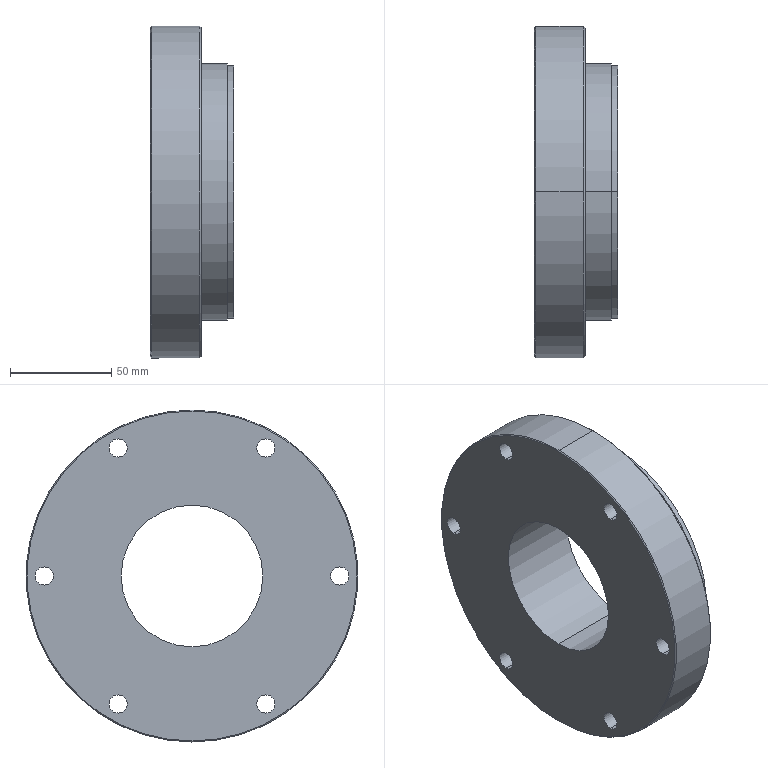Part | SolidWorks | features BaseBody 1 | 1 solid | 46 faces | box 41 x 164 x 164 mm | volume 556620 mm3 | cylinder 32 | plane 10 | cone 4 | commonest cylinder face diameters 9 x12 14 x12 70 x2 125 x2 127 x2 164 x2
STEP:
#1=CARTESIAN_POINT('',(41.,0.,-35.));
#2=VERTEX_POINT('',#1);
#3=CARTESIAN_POINT('',(41.,0.,35.));
#4=VERTEX_POINT('',#3);
#5=CARTESIAN_POINT('',(41.,0.,0.));
#6=DIRECTION('',(-1.,0.,0.));
#7=DIRECTION('',(0.,0.,1.));
#8=AXIS2_PLACEMENT_3D('',#5,#6,#7);
#9=CIRCLE('',#8,35.);
#10=EDGE_CURVE('',#2,#4,#9,.T.);
#11=ORIENTED_EDGE('',*,*,#10,.F.);
#12=CARTESIAN_POINT('',(0.,0.,-35.));
#13=VERTEX_POINT('',#12);
#14=CARTESIAN_POINT('',(-14.652,0.,-35.));
#15=DIRECTION('',(-1.,0.,0.));
#16=VECTOR('',#15,1000.);
#17=LINE('',#14,#16);
#18=EDGE_CURVE('',#2,#13,#17,.T.);
#19=ORIENTED_EDGE('',*,*,#18,.T.);
#20=CARTESIAN_POINT('',(0.,0.,35.));
#21=VERTEX_POINT('',#20);
#22=CARTESIAN_POINT('',(0.,0.,0.));
#23=DIRECTION('',(-1.,0.,0.));
#24=DIRECTION('',(0.,0.,1.));
#25=AXIS2_PLACEMENT_3D('',#22,#23,#24);
#26=CIRCLE('',#25,35.);
#27=EDGE_CURVE('',#13,#21,#26,.T.);
#28=ORIENTED_EDGE('',*,*,#27,.T.);
#29=CARTESIAN_POINT('',(-14.652,0.,35.));
#30=DIRECTION('',(-1.,0.,0.));
#31=VECTOR('',#30,1000.);
#32=LINE('',#29,#31);
#33=EDGE_CURVE('',#4,#21,#32,.T.);
#34=ORIENTED_EDGE('',*,*,#33,.F.);
#35=EDGE_LOOP('',(#11,#19,#28,#34));
#36=FACE_OUTER_BOUND('',#35,.T.);
#37=CARTESIAN_POINT('',(-14.652,0.,0.));
#38=DIRECTION('',(-1.,0.,0.));
#39=DIRECTION('',(0.,0.,1.));
#40=AXIS2_PLACEMENT_3D('',#37,#38,#39);
#41=CYLINDRICAL_SURFACE('',#40,35.);
#42=ADVANCED_FACE('',(#36),#41,.F.);
#43=CARTESIAN_POINT('',(0.,73.,-4.5));
#44=VERTEX_POINT('',#43);
#45=CARTESIAN_POINT('',(0.,73.,4.5));
#46=VERTEX_POINT('',#45);
#47=CARTESIAN_POINT('',(0.,73.,0.));
#48=DIRECTION('',(-1.,0.,0.));
#49=DIRECTION('',(0.,0.,-1.));
#50=AXIS2_PLACEMENT_3D('',#47,#48,#49);
#51=CIRCLE('',#50,4.5);
#52=EDGE_CURVE('',#44,#46,#51,.T.);
#53=ORIENTED_EDGE('',*,*,#52,.T.);
#54=CARTESIAN_POINT('',(15.,73.,4.5));
#55=VERTEX_POINT('',#54);
#56=CARTESIAN_POINT('',(25.,73.,4.5));
#57=DIRECTION('',(1.,0.,0.));
#58=VECTOR('',#57,1000.);
#59=LINE('',#56,#58);
#60=EDGE_CURVE('',#46,#55,#59,.T.);
#61=ORIENTED_EDGE('',*,*,#60,.T.);
#62=CARTESIAN_POINT('',(15.,73.,-4.5));
#63=VERTEX_POINT('',#62);
#64=CARTESIAN_POINT('',(15.,73.,0.));
#65=DIRECTION('',(-1.,0.,0.));
#66=DIRECTION('',(0.,0.,-1.));
#67=AXIS2_PLACEMENT_3D('',#64,#65,#66);
#68=CIRCLE('',#67,4.5);
#69=EDGE_CURVE('',#63,#55,#68,.T.);
#70=ORIENTED_EDGE('',*,*,#69,.F.);
#71=CARTESIAN_POINT('',(25.,73.,-4.5));
#72=DIRECTION('',(1.,0.,0.));
#73=VECTOR('',#72,1000.);
#74=LINE('',#71,#73);
#75=EDGE_CURVE('',#44,#63,#74,.T.);
#76=ORIENTED_EDGE('',*,*,#75,.F.);
#77=EDGE_LOOP('',(#53,#61,#70,#76));
#78=FACE_OUTER_BOUND('',#77,.T.);
#79=CARTESIAN_POINT('',(25.,73.,0.));
#80=DIRECTION('',(1.,0.,0.));
#81=DIRECTION('',(0.,0.,-1.));
#82=AXIS2_PLACEMENT_3D('',#79,#80,#81);
#83=CYLINDRICAL_SURFACE('',#82,4.5);
#84=ADVANCED_FACE('',(#78),#83,.F.);
#85=CARTESIAN_POINT('',(0.,36.5,-67.72));
#86=VERTEX_POINT('',#85);
#87=CARTESIAN_POINT('',(0.,36.5,-58.72));
#88=VERTEX_POINT('',#87);
#89=CARTESIAN_POINT('',(0.,36.5,-63.22));
#90=DIRECTION('',(-1.,0.,0.));
#91=DIRECTION('',(0.,0.,-1.));
#92=AXIS2_PLACEMENT_3D('',#89,#90,#91);
#93=CIRCLE('',#92,4.5);
#94=EDGE_CURVE('',#86,#88,#93,.T.);
#95=ORIENTED_EDGE('',*,*,#94,.T.);
#96=CARTESIAN_POINT('',(15.,36.5,-58.72));
#97=VERTEX_POINT('',#96);
#98=CARTESIAN_POINT('',(25.,36.5,-58.72));
#99=DIRECTION('',(1.,0.,0.));
#100=VECTOR('',#99,1000.);
#101=LINE('',#98,#100);
#102=EDGE_CURVE('',#88,#97,#101,.T.);
#103=ORIENTED_EDGE('',*,*,#102,.T.);
#104=CARTESIAN_POINT('',(15.,36.5,-67.72));
#105=VERTEX_POINT('',#104);
#106=CARTESIAN_POINT('',(15.,36.5,-63.22));
#107=DIRECTION('',(-1.,0.,0.));
#108=DIRECTION('',(0.,0.,-1.));
#109=AXIS2_PLACEMENT_3D('',#106,#107,#108);
#110=CIRCLE('',#109,4.5);
#111=EDGE_CURVE('',#105,#97,#110,.T.);
#112=ORIENTED_EDGE('',*,*,#111,.F.);
#113=CARTESIAN_POINT('',(25.,36.5,-67.72));
#114=DIRECTION('',(1.,0.,0.));
#115=VECTOR('',#114,1000.);
#116=LINE('',#113,#115);
#117=EDGE_CURVE('',#86,#105,#116,.T.);
#118=ORIENTED_EDGE('',*,*,#117,.F.);
#119=EDGE_LOOP('',(#95,#103,#112,#118));
#120=FACE_OUTER_BOUND('',#119,.T.);
#121=CARTESIAN_POINT('',(25.,36.5,-63.22));
#122=DIRECTION('',(1.,0.,0.));
#123=DIRECTION('',(0.,0.,-1.));
#124=AXIS2_PLACEMENT_3D('',#121,#122,#123);
#125=CYLINDRICAL_SURFACE('',#124,4.5);
#126=ADVANCED_FACE('',(#120),#125,.F.);
#127=CARTESIAN_POINT('',(0.,-36.5,-67.72));
#128=VERTEX_POINT('',#127);
#129=CARTESIAN_POINT('',(0.,-36.5,-58.72));
#130=VERTEX_POINT('',#129);
#131=CARTESIAN_POINT('',(0.,-36.5,-63.22));
#132=DIRECTION('',(-1.,0.,0.));
#133=DIRECTION('',(0.,0.,-1.));
#134=AXIS2_PLACEMENT_3D('',#131,#132,#133);
#135=CIRCLE('',#134,4.5);
#136=EDGE_CURVE('',#128,#130,#135,.T.);
#137=ORIENTED_EDGE('',*,*,#136,.T.);
#138=CARTESIAN_POINT('',(15.,-36.5,-58.72));
#139=VERTEX_POINT('',#138);
#140=CARTESIAN_POINT('',(25.,-36.5,-58.72));
#141=DIRECTION('',(1.,0.,0.));
#142=VECTOR('',#141,1000.);
#143=LINE('',#140,#142);
#144=EDGE_CURVE('',#130,#139,#143,.T.);
#145=ORIENTED_EDGE('',*,*,#144,.T.);
#146=CARTESIAN_POINT('',(15.,-36.5,-67.72));
#147=VERTEX_POINT('',#146);
#148=CARTESIAN_POINT('',(15.,-36.5,-63.22));
#149=DIRECTION('',(-1.,0.,0.));
#150=DIRECTION('',(0.,0.,-1.));
#151=AXIS2_PLACEMENT_3D('',#148,#149,#150);
#152=CIRCLE('',#151,4.5);
#153=EDGE_CURVE('',#147,#139,#152,.T.);
#154=ORIENTED_EDGE('',*,*,#153,.F.);
#155=CARTESIAN_POINT('',(25.,-36.5,-67.72));
#156=DIRECTION('',(1.,0.,0.));
#157=VECTOR('',#156,1000.);
#158=LINE('',#155,#157);
#159=EDGE_CURVE('',#128,#147,#158,.T.);
#160=ORIENTED_EDGE('',*,*,#159,.F.);
#161=EDGE_LOOP('',(#137,#145,#154,#160));
#162=FACE_OUTER_BOUND('',#161,.T.);
#163=CARTESIAN_POINT('',(25.,-36.5,-63.22));
#164=DIRECTION('',(1.,0.,0.));
#165=DIRECTION('',(0.,0.,-1.));
#166=AXIS2_PLACEMENT_3D('',#163,#164,#165);
#167=CYLINDRICAL_SURFACE('',#166,4.5);
#168=ADVANCED_FACE('',(#162),#167,.F.);
#169=CARTESIAN_POINT('',(0.,-73.,-4.5));
#170=VERTEX_POINT('',#169);
#171=CARTESIAN_POINT('',(0.,-73.,4.5));
#172=VERTEX_POINT('',#171);
#173=CARTESIAN_POINT('',(0.,-73.,0.));
#174=DIRECTION('',(-1.,0.,0.));
#175=DIRECTION('',(0.,0.,-1.));
#176=AXIS2_PLACEMENT_3D('',#173,#174,#175);
#177=CIRCLE('',#176,4.5);
#178=EDGE_CURVE('',#170,#172,#177,.T.);
#179=ORIENTED_EDGE('',*,*,#178,.T.);
#180=CARTESIAN_POINT('',(15.,-73.,4.5));
#181=VERTEX_POINT('',#180);
#182=CARTESIAN_POINT('',(25.,-73.,4.5));
#183=DIRECTION('',(1.,0.,0.));
#184=VECTOR('',#183,1000.);
#185=LINE('',#182,#184);
#186=EDGE_CURVE('',#172,#181,#185,.T.);
#187=ORIENTED_EDGE('',*,*,#186,.T.);
#188=CARTESIAN_POINT('',(15.,-73.,-4.5));
#189=VERTEX_POINT('',#188);
#190=CARTESIAN_POINT('',(15.,-73.,0.));
#191=DIRECTION('',(-1.,0.,0.));
#192=DIRECTION('',(0.,0.,-1.));
#193=AXIS2_PLACEMENT_3D('',#190,#191,#192);
#194=CIRCLE('',#193,4.5);
#195=EDGE_CURVE('',#189,#181,#194,.T.);
#196=ORIENTED_EDGE('',*,*,#195,.F.);
#197=CARTESIAN_POINT('',(25.,-73.,-4.5));
#198=DIRECTION('',(1.,0.,0.));
#199=VECTOR('',#198,1000.);
#200=LINE('',#197,#199);
#201=EDGE_CURVE('',#170,#189,#200,.T.);
#202=ORIENTED_EDGE('',*,*,#201,.F.);
#203=EDGE_LOOP('',(#179,#187,#196,#202));
#204=FACE_OUTER_BOUND('',#203,.T.);
#205=CARTESIAN_POINT('',(25.,-73.,0.));
#206=DIRECTION('',(1.,0.,0.));
#207=DIRECTION('',(0.,0.,-1.));
#208=AXIS2_PLACEMENT_3D('',#205,#206,#207);
#209=CYLINDRICAL_SURFACE('',#208,4.5);
#210=ADVANCED_FACE('',(#204),#209,.F.);
#211=CARTESIAN_POINT('',(0.,-36.5,58.72));
#212=VERTEX_POINT('',#211);
#213=CARTESIAN_POINT('',(0.,-36.5,67.72));
#214=VERTEX_POINT('',#213);
#215=CARTESIAN_POINT('',(0.,-36.5,63.22));
#216=DIRECTION('',(-1.,0.,0.));
#217=DIRECTION('',(0.,0.,-1.));
#218=AXIS2_PLACEMENT_3D('',#215,#216,#217);
#219=CIRCLE('',#218,4.5);
#220=EDGE_CURVE('',#212,#214,#219,.T.);
#221=ORIENTED_EDGE('',*,*,#220,.T.);
#222=CARTESIAN_POINT('',(15.,-36.5,67.72));
#223=VERTEX_POINT('',#222);
#224=CARTESIAN_POINT('',(25.,-36.5,67.72));
#225=DIRECTION('',(1.,0.,0.));
#226=VECTOR('',#225,1000.);
#227=LINE('',#224,#226);
#228=EDGE_CURVE('',#214,#223,#227,.T.);
#229=ORIENTED_EDGE('',*,*,#228,.T.);
#230=CARTESIAN_POINT('',(15.,-36.5,58.72));
#231=VERTEX_POINT('',#230);
#232=CARTESIAN_POINT('',(15.,-36.5,63.22));
#233=DIRECTION('',(-1.,0.,0.));
#234=DIRECTION('',(0.,0.,-1.));
#235=AXIS2_PLACEMENT_3D('',#232,#233,#234);
#236=CIRCLE('',#235,4.5);
#237=EDGE_CURVE('',#231,#223,#236,.T.);
#238=ORIENTED_EDGE('',*,*,#237,.F.);
#239=CARTESIAN_POINT('',(25.,-36.5,58.72));
#240=DIRECTION('',(1.,0.,0.));
#241=VECTOR('',#240,1000.);
#242=LINE('',#239,#241);
#243=EDGE_CURVE('',#212,#231,#242,.T.);
#244=ORIENTED_EDGE('',*,*,#243,.F.);
#245=EDGE_LOOP('',(#221,#229,#238,#244));
#246=FACE_OUTER_BOUND('',#245,.T.);
#247=CARTESIAN_POINT('',(25.,-36.5,63.22));
#248=DIRECTION('',(1.,0.,0.));
#249=DIRECTION('',(0.,0.,-1.));
#250=AXIS2_PLACEMENT_3D('',#247,#248,#249);
#251=CYLINDRICAL_SURFACE('',#250,4.5);
#252=ADVANCED_FACE('',(#246),#251,.F.);
#253=CARTESIAN_POINT('',(0.,36.5,58.72));
#254=VERTEX_POINT('',#253);
#255=CARTESIAN_POINT('',(0.,36.5,67.72));
#256=VERTEX_POINT('',#255);
#257=CARTESIAN_POINT('',(0.,36.5,63.22));
#258=DIRECTION('',(-1.,0.,0.));
#259=DIRECTION('',(0.,0.,-1.));
#260=AXIS2_PLACEMENT_3D('',#257,#258,#259);
#261=CIRCLE('',#260,4.5);
#262=EDGE_CURVE('',#254,#256,#261,.T.);
#263=ORIENTED_EDGE('',*,*,#262,.T.);
#264=CARTESIAN_POINT('',(15.,36.5,67.72));
#265=VERTEX_POINT('',#264);
#266=CARTESIAN_POINT('',(25.,36.5,67.72));
#267=DIRECTION('',(1.,0.,0.));
#268=VECTOR('',#267,1000.);
#269=LINE('',#266,#268);
#270=EDGE_CURVE('',#256,#265,#269,.T.);
#271=ORIENTED_EDGE('',*,*,#270,.T.);
#272=CARTESIAN_POINT('',(15.,36.5,58.72));
#273=VERTEX_POINT('',#272);
#274=CARTESIAN_POINT('',(15.,36.5,63.22));
#275=DIRECTION('',(-1.,0.,0.));
#276=DIRECTION('',(0.,0.,-1.));
#277=AXIS2_PLACEMENT_3D('',#274,#275,#276);
#278=CIRCLE('',#277,4.5);
#279=EDGE_CURVE('',#273,#265,#278,.T.);
#280=ORIENTED_EDGE('',*,*,#279,.F.);
#281=CARTESIAN_POINT('',(25.,36.5,58.72));
#282=DIRECTION('',(1.,0.,0.));
#283=VECTOR('',#282,1000.);
#284=LINE('',#281,#283);
#285=EDGE_CURVE('',#254,#273,#284,.T.);
#286=ORIENTED_EDGE('',*,*,#285,.F.);
#287=EDGE_LOOP('',(#263,#271,#280,#286));
#288=FACE_OUTER_BOUND('',#287,.T.);
#289=CARTESIAN_POINT('',(25.,36.5,63.22));
#290=DIRECTION('',(1.,0.,0.));
#291=DIRECTION('',(0.,0.,-1.));
#292=AXIS2_PLACEMENT_3D('',#289,#290,#291);
#293=CYLINDRICAL_SURFACE('',#292,4.5);
#294=ADVANCED_FACE('',(#288),#293,.F.);
#295=CARTESIAN_POINT('',(0.,0.,-81.5));
#296=VERTEX_POINT('',#295);
#297=CARTESIAN_POINT('',(0.,0.,81.5));
#298=VERTEX_POINT('',#297);
#299=CARTESIAN_POINT('',(0.,0.,0.));
#300=DIRECTION('',(1.,0.,0.));
#301=DIRECTION('',(0.,0.,-1.));
#302=AXIS2_PLACEMENT_3D('',#299,#300,#301);
#303=CIRCLE('',#302,81.5);
#304=EDGE_CURVE('',#296,#298,#303,.T.);
#305=ORIENTED_EDGE('',*,*,#304,.T.);
#306=CARTESIAN_POINT('',(0.5,0.,82.));
#307=VERTEX_POINT('',#306);
#308=CARTESIAN_POINT('',(0.5,0.,82.));
#309=DIRECTION('',(0.7071,0.,0.7071));
#310=VECTOR('',#309,1000.);
#311=LINE('',#308,#310);
#312=EDGE_CURVE('',#298,#307,#311,.T.);
#313=ORIENTED_EDGE('',*,*,#312,.T.);
#314=CARTESIAN_POINT('',(0.5,0.,-82.));
#315=VERTEX_POINT('',#314);
#316=CARTESIAN_POINT('',(0.5,0.,0.));
#317=DIRECTION('',(-1.,0.,0.));
#318=DIRECTION('',(0.,0.,-1.));
#319=AXIS2_PLACEMENT_3D('',#316,#317,#318);
#320=CIRCLE('',#319,82.);
#321=EDGE_CURVE('',#307,#315,#320,.T.);
#322=ORIENTED_EDGE('',*,*,#321,.T.);
#323=CARTESIAN_POINT('',(0.5,0.,-82.));
#324=DIRECTION('',(0.7071,0.,-0.7071));
#325=VECTOR('',#324,1000.);
#326=LINE('',#323,#325);
#327=EDGE_CURVE('',#296,#315,#326,.T.);
#328=ORIENTED_EDGE('',*,*,#327,.F.);
#329=EDGE_LOOP('',(#305,#313,#322,#328));
#330=FACE_OUTER_BOUND('',#329,.T.);
#331=CARTESIAN_POINT('',(0.5,0.,0.));
#332=DIRECTION('',(1.,0.,0.));
#333=DIRECTION('',(0.,0.,-1.));
#334=AXIS2_PLACEMENT_3D('',#331,#332,#333);
#335=CONICAL_SURFACE('',#334,82.,0.7854);
#336=ADVANCED_FACE('',(#330),#335,.T.);
#337=CARTESIAN_POINT('',(24.2,0.,82.));
#338=VERTEX_POINT('',#337);
#339=CARTESIAN_POINT('',(24.2,0.,-82.));
#340=VERTEX_POINT('',#339);
#341=CARTESIAN_POINT('',(24.2,0.,0.));
#342=DIRECTION('',(-1.,0.,0.));
#343=DIRECTION('',(0.,0.,1.));
#344=AXIS2_PLACEMENT_3D('',#341,#342,#343);
#345=CIRCLE('',#344,82.);
#346=EDGE_CURVE('',#338,#340,#345,.T.);
#347=ORIENTED_EDGE('',*,*,#346,.T.);
#348=CARTESIAN_POINT('',(-14.652,0.,-82.));
#349=DIRECTION('',(-1.,0.,0.));
#350=VECTOR('',#349,1000.);
#351=LINE('',#348,#350);
#352=EDGE_CURVE('',#340,#315,#351,.T.);
#353=ORIENTED_EDGE('',*,*,#352,.T.);
#354=ORIENTED_EDGE('',*,*,#321,.F.);
#355=CARTESIAN_POINT('',(-14.652,0.,82.));
#356=DIRECTION('',(-1.,0.,0.));
#357=VECTOR('',#356,1000.);
#358=LINE('',#355,#357);
#359=EDGE_CURVE('',#338,#307,#358,.T.);
#360=ORIENTED_EDGE('',*,*,#359,.F.);
#361=EDGE_LOOP('',(#347,#353,#354,#360));
#362=FACE_OUTER_BOUND('',#361,.T.);
#363=CARTESIAN_POINT('',(-14.652,0.,0.));
#364=DIRECTION('',(-1.,0.,0.));
#365=DIRECTION('',(0.,0.,1.));
#366=AXIS2_PLACEMENT_3D('',#363,#364,#365);
#367=CYLINDRICAL_SURFACE('',#366,82.);
#368=ADVANCED_FACE('',(#362),#367,.T.);
#369=CARTESIAN_POINT('',(41.,0.,62.5));
#370=VERTEX_POINT('',#369);
#371=CARTESIAN_POINT('',(41.,0.,-62.5));
#372=VERTEX_POINT('',#371);
#373=CARTESIAN_POINT('',(41.,0.,0.));
#374=DIRECTION('',(-1.,0.,0.));
#375=DIRECTION('',(0.,0.,1.));
#376=AXIS2_PLACEMENT_3D('',#373,#374,#375);
#377=CIRCLE('',#376,62.5);
#378=EDGE_CURVE('',#370,#372,#377,.T.);
#379=ORIENTED_EDGE('',*,*,#378,.T.);
#380=CARTESIAN_POINT('',(38.,0.,-62.5));
#381=VERTEX_POINT('',#380);
#382=CARTESIAN_POINT('',(-14.652,0.,-62.5));
#383=DIRECTION('',(-1.,0.,0.));
#384=VECTOR('',#383,1000.);
#385=LINE('',#382,#384);
#386=EDGE_CURVE('',#372,#381,#385,.T.);
#387=ORIENTED_EDGE('',*,*,#386,.T.);
#388=CARTESIAN_POINT('',(38.,0.,62.5));
#389=VERTEX_POINT('',#388);
#390=CARTESIAN_POINT('',(38.,0.,0.));
#391=DIRECTION('',(1.,0.,0.));
#392=DIRECTION('',(0.,0.,1.));
#393=AXIS2_PLACEMENT_3D('',#390,#391,#392);
#394=CIRCLE('',#393,62.5);
#395=EDGE_CURVE('',#381,#389,#394,.T.);
#396=ORIENTED_EDGE('',*,*,#395,.T.);
#397=CARTESIAN_POINT('',(-14.652,0.,62.5));
#398=DIRECTION('',(-1.,0.,0.));
#399=VECTOR('',#398,1000.);
#400=LINE('',#397,#399);
#401=EDGE_CURVE('',#370,#389,#400,.T.);
#402=ORIENTED_EDGE('',*,*,#401,.F.);
#403=EDGE_LOOP('',(#379,#387,#396,#402));
#404=FACE_OUTER_BOUND('',#403,.T.);
#405=CARTESIAN_POINT('',(-14.652,0.,0.));
#406=DIRECTION('',(-1.,0.,0.));
#407=DIRECTION('',(0.,0.,1.));
#408=AXIS2_PLACEMENT_3D('',#405,#406,#407);
#409=CYLINDRICAL_SURFACE('',#408,62.5);
#410=ADVANCED_FACE('',(#404),#409,.T.);
#411=CARTESIAN_POINT('',(15.,73.,-7.));
#412=VERTEX_POINT('',#411);
#413=CARTESIAN_POINT('',(15.,73.,7.));
#414=VERTEX_POINT('',#413);
#415=CARTESIAN_POINT('',(15.,73.,0.));
#416=DIRECTION('',(-1.,0.,0.));
#417=DIRECTION('',(0.,0.,-1.));
#418=AXIS2_PLACEMENT_3D('',#415,#416,#417);
#419=CIRCLE('',#418,7.);
#420=EDGE_CURVE('',#412,#414,#419,.T.);
#421=ORIENTED_EDGE('',*,*,#420,.T.);
#422=CARTESIAN_POINT('',(25.,73.,7.));
#423=VERTEX_POINT('',#422);
#424=CARTESIAN_POINT('',(25.,73.,7.));
#425=DIRECTION('',(1.,0.,0.));
#426=VECTOR('',#425,1000.);
#427=LINE('',#424,#426);
#428=EDGE_CURVE('',#414,#423,#427,.T.);
#429=ORIENTED_EDGE('',*,*,#428,.T.);
#430=CARTESIAN_POINT('',(25.,73.,-7.));
#431=VERTEX_POINT('',#430);
#432=CARTESIAN_POINT('',(25.,73.,0.));
#433=DIRECTION('',(-1.,0.,0.));
#434=DIRECTION('',(0.,0.,-1.));
#435=AXIS2_PLACEMENT_3D('',#432,#433,#434);
#436=CIRCLE('',#435,7.);
#437=EDGE_CURVE('',#431,#423,#436,.T.);
#438=ORIENTED_EDGE('',*,*,#437,.F.);
#439=CARTESIAN_POINT('',(25.,73.,-7.));
#440=DIRECTION('',(1.,0.,0.));
#441=VECTOR('',#440,1000.);
#442=LINE('',#439,#441);
#443=EDGE_CURVE('',#412,#431,#442,.T.);
#444=ORIENTED_EDGE('',*,*,#443,.F.);
#445=EDGE_LOOP('',(#421,#429,#438,#444));
#446=FACE_OUTER_BOUND('',#445,.T.);
#447=CARTESIAN_POINT('',(25.,73.,0.));
#448=DIRECTION('',(1.,0.,0.));
#449=DIRECTION('',(0.,0.,-1.));
#450=AXIS2_PLACEMENT_3D('',#447,#448,#449);
#451=CYLINDRICAL_SURFACE('',#450,7.);
#452=ADVANCED_FACE('',(#446),#451,.F.);
#453=CARTESIAN_POINT('',(15.,36.5,-70.22));
#454=VERTEX_POINT('',#453);
#455=CARTESIAN_POINT('',(15.,36.5,-56.22));
#456=VERTEX_POINT('',#455);
#457=CARTESIAN_POINT('',(15.,36.5,-63.22));
#458=DIRECTION('',(-1.,0.,0.));
#459=DIRECTION('',(0.,0.,-1.));
#460=AXIS2_PLACEMENT_3D('',#457,#458,#459);
#461=CIRCLE('',#460,7.);
#462=EDGE_CURVE('',#454,#456,#461,.T.);
#463=ORIENTED_EDGE('',*,*,#462,.T.);
#464=CARTESIAN_POINT('',(25.,36.5,-56.22));
#465=VERTEX_POINT('',#464);
#466=CARTESIAN_POINT('',(25.,36.5,-56.22));
#467=DIRECTION('',(1.,0.,0.));
#468=VECTOR('',#467,1000.);
#469=LINE('',#466,#468);
#470=EDGE_CURVE('',#456,#465,#469,.T.);
#471=ORIENTED_EDGE('',*,*,#470,.T.);
#472=CARTESIAN_POINT('',(25.,36.5,-70.22));
#473=VERTEX_POINT('',#472);
#474=CARTESIAN_POINT('',(25.,36.5,-63.22));
#475=DIRECTION('',(-1.,0.,0.));
#476=DIRECTION('',(0.,0.,-1.));
#477=AXIS2_PLACEMENT_3D('',#474,#475,#476);
#478=CIRCLE('',#477,7.);
#479=EDGE_CURVE('',#473,#465,#478,.T.);
#480=ORIENTED_EDGE('',*,*,#479,.F.);
#481=CARTESIAN_POINT('',(25.,36.5,-70.22));
#482=DIRECTION('',(1.,0.,0.));
#483=VECTOR('',#482,1000.);
#484=LINE('',#481,#483);
#485=EDGE_CURVE('',#454,#473,#484,.T.);
#486=ORIENTED_EDGE('',*,*,#485,.F.);
#487=EDGE_LOOP('',(#463,#471,#480,#486));
#488=FACE_OUTER_BOUND('',#487,.T.);
#489=CARTESIAN_POINT('',(25.,36.5,-63.22));
#490=DIRECTION('',(1.,0.,0.));
#491=DIRECTION('',(0.,0.,-1.));
#492=AXIS2_PLACEMENT_3D('',#489,#490,#491);
#493=CYLINDRICAL_SURFACE('',#492,7.);
#494=ADVANCED_FACE('',(#488),#493,.F.);
#495=CARTESIAN_POINT('',(15.,-36.5,-70.22));
#496=VERTEX_POINT('',#495);
#497=CARTESIAN_POINT('',(15.,-36.5,-56.22));
#498=VERTEX_POINT('',#497);
#499=CARTESIAN_POINT('',(15.,-36.5,-63.22));
#500=DIRECTION('',(-1.,0.,0.));
#501=DIRECTION('',(0.,0.,-1.));
#502=AXIS2_PLACEMENT_3D('',#499,#500,#501);
#503=CIRCLE('',#502,7.);
#504=EDGE_CURVE('',#496,#498,#503,.T.);
#505=ORIENTED_EDGE('',*,*,#504,.T.);
#506=CARTESIAN_POINT('',(25.,-36.5,-56.22));
#507=VERTEX_POINT('',#506);
#508=CARTESIAN_POINT('',(25.,-36.5,-56.22));
#509=DIRECTION('',(1.,0.,0.));
#510=VECTOR('',#509,1000.);
#511=LINE('',#508,#510);
#512=EDGE_CURVE('',#498,#507,#511,.T.);
#513=ORIENTED_EDGE('',*,*,#512,.T.);
#514=CARTESIAN_POINT('',(25.,-36.5,-70.22));
#515=VERTEX_POINT('',#514);
#516=CARTESIAN_POINT('',(25.,-36.5,-63.22));
#517=DIRECTION('',(-1.,0.,0.));
#518=DIRECTION('',(0.,0.,-1.));
#519=AXIS2_PLACEMENT_3D('',#516,#517,#518);
#520=CIRCLE('',#519,7.);
#521=EDGE_CURVE('',#515,#507,#520,.T.);
#522=ORIENTED_EDGE('',*,*,#521,.F.);
#523=CARTESIAN_POINT('',(25.,-36.5,-70.22));
#524=DIRECTION('',(1.,0.,0.));
#525=VECTOR('',#524,1000.);
#526=LINE('',#523,#525);
#527=EDGE_CURVE('',#496,#515,#526,.T.);
#528=ORIENTED_EDGE('',*,*,#527,.F.);
#529=EDGE_LOOP('',(#505,#513,#522,#528));
#530=FACE_OUTER_BOUND('',#529,.T.);
#531=CARTESIAN_POINT('',(25.,-36.5,-63.22));
#532=DIRECTION('',(1.,0.,0.));
#533=DIRECTION('',(0.,0.,-1.));
#534=AXIS2_PLACEMENT_3D('',#531,#532,#533);
#535=CYLINDRICAL_SURFACE('',#534,7.);
#536=ADVANCED_FACE('',(#530),#535,.F.);
#537=CARTESIAN_POINT('',(15.,-73.,-7.));
#538=VERTEX_POINT('',#537);
#539=CARTESIAN_POINT('',(15.,-73.,7.));
#540=VERTEX_POINT('',#539);
#541=CARTESIAN_POINT('',(15.,-73.,0.));
#542=DIRECTION('',(-1.,0.,0.));
#543=DIRECTION('',(0.,0.,-1.));
#544=AXIS2_PLACEMENT_3D('',#541,#542,#543);
#545=CIRCLE('',#544,7.);
#546=EDGE_CURVE('',#538,#540,#545,.T.);
#547=ORIENTED_EDGE('',*,*,#546,.T.);
#548=CARTESIAN_POINT('',(25.,-73.,7.));
#549=VERTEX_POINT('',#548);
#550=CARTESIAN_POINT('',(25.,-73.,7.));
#551=DIRECTION('',(1.,0.,0.));
#552=VECTOR('',#551,1000.);
#553=LINE('',#550,#552);
#554=EDGE_CURVE('',#540,#549,#553,.T.);
#555=ORIENTED_EDGE('',*,*,#554,.T.);
#556=CARTESIAN_POINT('',(25.,-73.,-7.));
#557=VERTEX_POINT('',#556);
#558=CARTESIAN_POINT('',(25.,-73.,0.));
#559=DIRECTION('',(-1.,0.,0.));
#560=DIRECTION('',(0.,0.,-1.));
#561=AXIS2_PLACEMENT_3D('',#558,#559,#560);
#562=CIRCLE('',#561,7.);
#563=EDGE_CURVE('',#557,#549,#562,.T.);
#564=ORIENTED_EDGE('',*,*,#563,.F.);
#565=CARTESIAN_POINT('',(25.,-73.,-7.));
#566=DIRECTION('',(1.,0.,0.));
#567=VECTOR('',#566,1000.);
#568=LINE('',#565,#567);
#569=EDGE_CURVE('',#538,#557,#568,.T.);
#570=ORIENTED_EDGE('',*,*,#569,.F.);
#571=EDGE_LOOP('',(#547,#555,#564,#570));
#572=FACE_OUTER_BOUND('',#571,.T.);
#573=CARTESIAN_POINT('',(25.,-73.,0.));
#574=DIRECTION('',(1.,0.,0.));
#575=DIRECTION('',(0.,0.,-1.));
#576=AXIS2_PLACEMENT_3D('',#573,#574,#575);
#577=CYLINDRICAL_SURFACE('',#576,7.);
#578=ADVANCED_FACE('',(#572),#577,.F.);
#579=CARTESIAN_POINT('',(15.,-36.5,56.22));
#580=VERTEX_POINT('',#579);
#581=CARTESIAN_POINT('',(15.,-36.5,70.22));
#582=VERTEX_POINT('',#581);
#583=CARTESIAN_POINT('',(15.,-36.5,63.22));
#584=DIRECTION('',(-1.,0.,0.));
#585=DIRECTION('',(0.,0.,-1.));
#586=AXIS2_PLACEMENT_3D('',#583,#584,#585);
#587=CIRCLE('',#586,7.);
#588=EDGE_CURVE('',#580,#582,#587,.T.);
#589=ORIENTED_EDGE('',*,*,#588,.T.);
#590=CARTESIAN_POINT('',(25.,-36.5,70.22));
#591=VERTEX_POINT('',#590);
#592=CARTESIAN_POINT('',(25.,-36.5,70.22));
#593=DIRECTION('',(1.,0.,0.));
#594=VECTOR('',#593,1000.);
#595=LINE('',#592,#594);
#596=EDGE_CURVE('',#582,#591,#595,.T.);
#597=ORIENTED_EDGE('',*,*,#596,.T.);
#598=CARTESIAN_POINT('',(25.,-36.5,56.22));
#599=VERTEX_POINT('',#598);
#600=CARTESIAN_POINT('',(25.,-36.5,63.22));
#601=DIRECTION('',(-1.,0.,0.));
#602=DIRECTION('',(0.,0.,-1.));
#603=AXIS2_PLACEMENT_3D('',#600,#601,#602);
#604=CIRCLE('',#603,7.);
#605=EDGE_CURVE('',#599,#591,#604,.T.);
#606=ORIENTED_EDGE('',*,*,#605,.F.);
#607=CARTESIAN_POINT('',(25.,-36.5,56.22));
#608=DIRECTION('',(1.,0.,0.));
#609=VECTOR('',#608,1000.);
#610=LINE('',#607,#609);
#611=EDGE_CURVE('',#580,#599,#610,.T.);
#612=ORIENTED_EDGE('',*,*,#611,.F.);
#613=EDGE_LOOP('',(#589,#597,#606,#612));
#614=FACE_OUTER_BOUND('',#613,.T.);
#615=CARTESIAN_POINT('',(25.,-36.5,63.22));
#616=DIRECTION('',(1.,0.,0.));
#617=DIRECTION('',(0.,0.,-1.));
#618=AXIS2_PLACEMENT_3D('',#615,#616,#617);
#619=CYLINDRICAL_SURFACE('',#618,7.);
#620=ADVANCED_FACE('',(#614),#619,.F.);
#621=CARTESIAN_POINT('',(15.,36.5,56.22));
#622=VERTEX_POINT('',#621);
#623=CARTESIAN_POINT('',(15.,36.5,70.22));
#624=VERTEX_POINT('',#623);
#625=CARTESIAN_POINT('',(15.,36.5,63.22));
#626=DIRECTION('',(-1.,0.,0.));
#627=DIRECTION('',(0.,0.,-1.));
#628=AXIS2_PLACEMENT_3D('',#625,#626,#627);
#629=CIRCLE('',#628,7.);
#630=EDGE_CURVE('',#622,#624,#629,.T.);
#631=ORIENTED_EDGE('',*,*,#630,.T.);
#632=CARTESIAN_POINT('',(25.,36.5,70.22));
#633=VERTEX_POINT('',#632);
#634=CARTESIAN_POINT('',(25.,36.5,70.22));
#635=DIRECTION('',(1.,0.,0.));
#636=VECTOR('',#635,1000.);
#637=LINE('',#634,#636);
#638=EDGE_CURVE('',#624,#633,#637,.T.);
#639=ORIENTED_EDGE('',*,*,#638,.T.);
#640=CARTESIAN_POINT('',(25.,36.5,56.22));
#641=VERTEX_POINT('',#640);
#642=CARTESIAN_POINT('',(25.,36.5,63.22));
#643=DIRECTION('',(-1.,0.,0.));
#644=DIRECTION('',(0.,0.,-1.));
#645=AXIS2_PLACEMENT_3D('',#642,#643,#644);
#646=CIRCLE('',#645,7.);
#647=EDGE_CURVE('',#641,#633,#646,.T.);
#648=ORIENTED_EDGE('',*,*,#647,.F.);
#649=CARTESIAN_POINT('',(25.,36.5,56.22));
#650=DIRECTION('',(1.,0.,0.));
#651=VECTOR('',#650,1000.);
#652=LINE('',#649,#651);
#653=EDGE_CURVE('',#622,#641,#652,.T.);
#654=ORIENTED_EDGE('',*,*,#653,.F.);
#655=EDGE_LOOP('',(#631,#639,#648,#654));
#656=FACE_OUTER_BOUND('',#655,.T.);
#657=CARTESIAN_POINT('',(25.,36.5,63.22));
#658=DIRECTION('',(1.,0.,0.));
#659=DIRECTION('',(0.,0.,-1.));
#660=AXIS2_PLACEMENT_3D('',#657,#658,#659);
#661=CYLINDRICAL_SURFACE('',#660,7.);
#662=ADVANCED_FACE('',(#656),#661,.F.);
#663=CARTESIAN_POINT('',(25.,0.,81.2));
#664=VERTEX_POINT('',#663);
#665=CARTESIAN_POINT('',(25.,0.,-81.2));
#666=VERTEX_POINT('',#665);
#667=CARTESIAN_POINT('',(25.,0.,0.));
#668=DIRECTION('',(-1.,0.,0.));
#669=DIRECTION('',(0.,0.,1.));
#670=AXIS2_PLACEMENT_3D('',#667,#668,#669);
#671=CIRCLE('',#670,81.2);
#672=EDGE_CURVE('',#664,#666,#671,.T.);
#673=ORIENTED_EDGE('',*,*,#672,.T.);
#674=CARTESIAN_POINT('',(24.2,0.,-82.));
#675=DIRECTION('',(-0.7071,0.,-0.7071));
#676=VECTOR('',#675,1000.);
#677=LINE('',#674,#676);
#678=EDGE_CURVE('',#666,#340,#677,.T.);
#679=ORIENTED_EDGE('',*,*,#678,.T.);
#680=ORIENTED_EDGE('',*,*,#346,.F.);
#681=CARTESIAN_POINT('',(24.2,0.,82.));
#682=DIRECTION('',(-0.7071,0.,0.7071));
#683=VECTOR('',#682,1000.);
#684=LINE('',#681,#683);
#685=EDGE_CURVE('',#664,#338,#684,.T.);
#686=ORIENTED_EDGE('',*,*,#685,.F.);
#687=EDGE_LOOP('',(#673,#679,#680,#686));
#688=FACE_OUTER_BOUND('',#687,.T.);
#689=CARTESIAN_POINT('',(24.2,0.,0.));
#690=DIRECTION('',(-1.,0.,0.));
#691=DIRECTION('',(0.,0.,1.));
#692=AXIS2_PLACEMENT_3D('',#689,#690,#691);
#693=CONICAL_SURFACE('',#692,82.,0.7854);
#694=ADVANCED_FACE('',(#688),#693,.T.);
#695=CARTESIAN_POINT('',(38.,0.,63.5));
#696=VERTEX_POINT('',#695);
#697=CARTESIAN_POINT('',(38.,0.,-63.5));
#698=VERTEX_POINT('',#697);
#699=CARTESIAN_POINT('',(38.,0.,0.));
#700=DIRECTION('',(-1.,0.,0.));
#701=DIRECTION('',(0.,0.,1.));
#702=AXIS2_PLACEMENT_3D('',#699,#700,#701);
#703=CIRCLE('',#702,63.5);
#704=EDGE_CURVE('',#696,#698,#703,.T.);
#705=ORIENTED_EDGE('',*,*,#704,.T.);
#706=CARTESIAN_POINT('',(25.,0.,-63.5));
#707=VERTEX_POINT('',#706);
#708=CARTESIAN_POINT('',(-14.652,0.,-63.5));
#709=DIRECTION('',(-1.,0.,0.));
#710=VECTOR('',#709,1000.);
#711=LINE('',#708,#710);
#712=EDGE_CURVE('',#698,#707,#711,.T.);
#713=ORIENTED_EDGE('',*,*,#712,.T.);
#714=CARTESIAN_POINT('',(25.,0.,63.5));
#715=VERTEX_POINT('',#714);
#716=CARTESIAN_POINT('',(25.,0.,0.));
#717=DIRECTION('',(1.,0.,0.));
#718=DIRECTION('',(0.,0.,1.));
#719=AXIS2_PLACEMENT_3D('',#716,#717,#718);
#720=CIRCLE('',#719,63.5);
#721=EDGE_CURVE('',#707,#715,#720,.T.);
#722=ORIENTED_EDGE('',*,*,#721,.T.);
#723=CARTESIAN_POINT('',(-14.652,0.,63.5));
#724=DIRECTION('',(-1.,0.,0.));
#725=VECTOR('',#724,1000.);
#726=LINE('',#723,#725);
#727=EDGE_CURVE('',#696,#715,#726,.T.);
#728=ORIENTED_EDGE('',*,*,#727,.F.);
#729=EDGE_LOOP('',(#705,#713,#722,#728));
#730=FACE_OUTER_BOUND('',#729,.T.);
#731=CARTESIAN_POINT('',(-14.652,0.,0.));
#732=DIRECTION('',(-1.,0.,0.));
#733=DIRECTION('',(0.,0.,1.));
#734=AXIS2_PLACEMENT_3D('',#731,#732,#733);
#735=CYLINDRICAL_SURFACE('',#734,63.5);
#736=ADVANCED_FACE('',(#730),#735,.T.);
#737=CARTESIAN_POINT('',(0.,0.,0.));
#738=DIRECTION('',(-1.,0.,0.));
#739=DIRECTION('',(0.,0.,1.));
#740=AXIS2_PLACEMENT_3D('',#737,#738,#739);
#741=CIRCLE('',#740,35.);
#742=EDGE_CURVE('',#21,#13,#741,.T.);
#743=ORIENTED_EDGE('',*,*,#742,.F.);
#744=ORIENTED_EDGE('',*,*,#27,.F.);
#745=EDGE_LOOP('',(#743,#744));
#746=FACE_BOUND('',#745,.T.);
#747=ORIENTED_EDGE('',*,*,#52,.F.);
#748=CARTESIAN_POINT('',(0.,73.,0.));
#749=DIRECTION('',(-1.,0.,0.));
#750=DIRECTION('',(0.,0.,-1.));
#751=AXIS2_PLACEMENT_3D('',#748,#749,#750);
#752=CIRCLE('',#751,4.5);
#753=EDGE_CURVE('',#46,#44,#752,.T.);
#754=ORIENTED_EDGE('',*,*,#753,.F.);
#755=EDGE_LOOP('',(#747,#754));
#756=FACE_BOUND('',#755,.T.);
#757=ORIENTED_EDGE('',*,*,#94,.F.);
#758=CARTESIAN_POINT('',(0.,36.5,-63.22));
#759=DIRECTION('',(-1.,0.,0.));
#760=DIRECTION('',(0.,0.,-1.));
#761=AXIS2_PLACEMENT_3D('',#758,#759,#760);
#762=CIRCLE('',#761,4.5);
#763=EDGE_CURVE('',#88,#86,#762,.T.);
#764=ORIENTED_EDGE('',*,*,#763,.F.);
#765=EDGE_LOOP('',(#757,#764));
#766=FACE_BOUND('',#765,.T.);
#767=ORIENTED_EDGE('',*,*,#136,.F.);
#768=CARTESIAN_POINT('',(0.,-36.5,-63.22));
#769=DIRECTION('',(-1.,0.,0.));
#770=DIRECTION('',(0.,0.,-1.));
#771=AXIS2_PLACEMENT_3D('',#768,#769,#770);
#772=CIRCLE('',#771,4.5);
#773=EDGE_CURVE('',#130,#128,#772,.T.);
#774=ORIENTED_EDGE('',*,*,#773,.F.);
#775=EDGE_LOOP('',(#767,#774));
#776=FACE_BOUND('',#775,.T.);
#777=ORIENTED_EDGE('',*,*,#178,.F.);
#778=CARTESIAN_POINT('',(0.,-73.,0.));
#779=DIRECTION('',(-1.,0.,0.));
#780=DIRECTION('',(0.,0.,-1.));
#781=AXIS2_PLACEMENT_3D('',#778,#779,#780);
#782=CIRCLE('',#781,4.5);
#783=EDGE_CURVE('',#172,#170,#782,.T.);
#784=ORIENTED_EDGE('',*,*,#783,.F.);
#785=EDGE_LOOP('',(#777,#784));
#786=FACE_BOUND('',#785,.T.);
#787=ORIENTED_EDGE('',*,*,#220,.F.);
#788=CARTESIAN_POINT('',(0.,-36.5,63.22));
#789=DIRECTION('',(-1.,0.,0.));
#790=DIRECTION('',(0.,0.,-1.));
#791=AXIS2_PLACEMENT_3D('',#788,#789,#790);
#792=CIRCLE('',#791,4.5);
#793=EDGE_CURVE('',#214,#212,#792,.T.);
#794=ORIENTED_EDGE('',*,*,#793,.F.);
#795=EDGE_LOOP('',(#787,#794));
#796=FACE_BOUND('',#795,.T.);
#797=ORIENTED_EDGE('',*,*,#262,.F.);
#798=CARTESIAN_POINT('',(0.,36.5,63.22));
#799=DIRECTION('',(-1.,0.,0.));
#800=DIRECTION('',(0.,0.,-1.));
#801=AXIS2_PLACEMENT_3D('',#798,#799,#800);
#802=CIRCLE('',#801,4.5);
#803=EDGE_CURVE('',#256,#254,#802,.T.);
#804=ORIENTED_EDGE('',*,*,#803,.F.);
#805=EDGE_LOOP('',(#797,#804));
#806=FACE_BOUND('',#805,.T.);
#807=ORIENTED_EDGE('',*,*,#304,.F.);
#808=CARTESIAN_POINT('',(0.,0.,0.));
#809=DIRECTION('',(1.,0.,0.));
#810=DIRECTION('',(0.,0.,-1.));
#811=AXIS2_PLACEMENT_3D('',#808,#809,#810);
#812=CIRCLE('',#811,81.5);
#813=EDGE_CURVE('',#298,#296,#812,.T.);
#814=ORIENTED_EDGE('',*,*,#813,.F.);
#815=EDGE_LOOP('',(#807,#814));
#816=FACE_OUTER_BOUND('',#815,.T.);
#817=CARTESIAN_POINT('',(0.,35.,0.));
#818=DIRECTION('',(1.,0.,0.));
#819=DIRECTION('',(0.,0.,-1.));
#820=AXIS2_PLACEMENT_3D('',#817,#818,#819);
#821=PLANE('',#820);
#822=ADVANCED_FACE('',(#746,#756,#766,#776,#786,#796,#806,#816),#821,.F.);
#823=ORIENTED_EDGE('',*,*,#18,.F.);
#824=CARTESIAN_POINT('',(41.,0.,0.));
#825=DIRECTION('',(-1.,0.,0.));
#826=DIRECTION('',(0.,0.,1.));
#827=AXIS2_PLACEMENT_3D('',#824,#825,#826);
#828=CIRCLE('',#827,35.);
#829=EDGE_CURVE('',#4,#2,#828,.T.);
#830=ORIENTED_EDGE('',*,*,#829,.F.);
#831=ORIENTED_EDGE('',*,*,#33,.T.);
#832=ORIENTED_EDGE('',*,*,#742,.T.);
#833=EDGE_LOOP('',(#823,#830,#831,#832));
#834=FACE_OUTER_BOUND('',#833,.T.);
#835=CARTESIAN_POINT('',(-14.652,0.,0.));
#836=DIRECTION('',(-1.,0.,0.));
#837=DIRECTION('',(0.,0.,1.));
#838=AXIS2_PLACEMENT_3D('',#835,#836,#837);
#839=CYLINDRICAL_SURFACE('',#838,35.);
#840=ADVANCED_FACE('',(#834),#839,.F.);
#841=ORIENTED_EDGE('',*,*,#60,.F.);
#842=ORIENTED_EDGE('',*,*,#753,.T.);
#843=ORIENTED_EDGE('',*,*,#75,.T.);
#844=CARTESIAN_POINT('',(15.,73.,0.));
#845=DIRECTION('',(-1.,0.,0.));
#846=DIRECTION('',(0.,0.,-1.));
#847=AXIS2_PLACEMENT_3D('',#844,#845,#846);
#848=CIRCLE('',#847,4.5);
#849=EDGE_CURVE('',#55,#63,#848,.T.);
#850=ORIENTED_EDGE('',*,*,#849,.F.);
#851=EDGE_LOOP('',(#841,#842,#843,#850));
#852=FACE_OUTER_BOUND('',#851,.T.);
#853=CARTESIAN_POINT('',(25.,73.,0.));
#854=DIRECTION('',(1.,0.,0.));
#855=DIRECTION('',(0.,0.,-1.));
#856=AXIS2_PLACEMENT_3D('',#853,#854,#855);
#857=CYLINDRICAL_SURFACE('',#856,4.5);
#858=ADVANCED_FACE('',(#852),#857,.F.);
#859=ORIENTED_EDGE('',*,*,#102,.F.);
#860=ORIENTED_EDGE('',*,*,#763,.T.);
#861=ORIENTED_EDGE('',*,*,#117,.T.);
#862=CARTESIAN_POINT('',(15.,36.5,-63.22));
#863=DIRECTION('',(-1.,0.,0.));
#864=DIRECTION('',(0.,0.,-1.));
#865=AXIS2_PLACEMENT_3D('',#862,#863,#864);
#866=CIRCLE('',#865,4.5);
#867=EDGE_CURVE('',#97,#105,#866,.T.);
#868=ORIENTED_EDGE('',*,*,#867,.F.);
#869=EDGE_LOOP('',(#859,#860,#861,#868));
#870=FACE_OUTER_BOUND('',#869,.T.);
#871=CARTESIAN_POINT('',(25.,36.5,-63.22));
#872=DIRECTION('',(1.,0.,0.));
#873=DIRECTION('',(0.,0.,-1.));
#874=AXIS2_PLACEMENT_3D('',#871,#872,#873);
#875=CYLINDRICAL_SURFACE('',#874,4.5);
#876=ADVANCED_FACE('',(#870),#875,.F.);
#877=ORIENTED_EDGE('',*,*,#144,.F.);
#878=ORIENTED_EDGE('',*,*,#773,.T.);
#879=ORIENTED_EDGE('',*,*,#159,.T.);
#880=CARTESIAN_POINT('',(15.,-36.5,-63.22));
#881=DIRECTION('',(-1.,0.,0.));
#882=DIRECTION('',(0.,0.,-1.));
#883=AXIS2_PLACEMENT_3D('',#880,#881,#882);
#884=CIRCLE('',#883,4.5);
#885=EDGE_CURVE('',#139,#147,#884,.T.);
#886=ORIENTED_EDGE('',*,*,#885,.F.);
#887=EDGE_LOOP('',(#877,#878,#879,#886));
#888=FACE_OUTER_BOUND('',#887,.T.);
#889=CARTESIAN_POINT('',(25.,-36.5,-63.22));
#890=DIRECTION('',(1.,0.,0.));
#891=DIRECTION('',(0.,0.,-1.));
#892=AXIS2_PLACEMENT_3D('',#889,#890,#891);
#893=CYLINDRICAL_SURFACE('',#892,4.5);
#894=ADVANCED_FACE('',(#888),#893,.F.);
#895=ORIENTED_EDGE('',*,*,#186,.F.);
#896=ORIENTED_EDGE('',*,*,#783,.T.);
#897=ORIENTED_EDGE('',*,*,#201,.T.);
#898=CARTESIAN_POINT('',(15.,-73.,0.));
#899=DIRECTION('',(-1.,0.,0.));
#900=DIRECTION('',(0.,0.,-1.));
#901=AXIS2_PLACEMENT_3D('',#898,#899,#900);
#902=CIRCLE('',#901,4.5);
#903=EDGE_CURVE('',#181,#189,#902,.T.);
#904=ORIENTED_EDGE('',*,*,#903,.F.);
#905=EDGE_LOOP('',(#895,#896,#897,#904));
#906=FACE_OUTER_BOUND('',#905,.T.);
#907=CARTESIAN_POINT('',(25.,-73.,0.));
#908=DIRECTION('',(1.,0.,0.));
#909=DIRECTION('',(0.,0.,-1.));
#910=AXIS2_PLACEMENT_3D('',#907,#908,#909);
#911=CYLINDRICAL_SURFACE('',#910,4.5);
#912=ADVANCED_FACE('',(#906),#911,.F.);
#913=ORIENTED_EDGE('',*,*,#228,.F.);
#914=ORIENTED_EDGE('',*,*,#793,.T.);
#915=ORIENTED_EDGE('',*,*,#243,.T.);
#916=CARTESIAN_POINT('',(15.,-36.5,63.22));
#917=DIRECTION('',(-1.,0.,0.));
#918=DIRECTION('',(0.,0.,-1.));
#919=AXIS2_PLACEMENT_3D('',#916,#917,#918);
#920=CIRCLE('',#919,4.5);
#921=EDGE_CURVE('',#223,#231,#920,.T.);
#922=ORIENTED_EDGE('',*,*,#921,.F.);
#923=EDGE_LOOP('',(#913,#914,#915,#922));
#924=FACE_OUTER_BOUND('',#923,.T.);
#925=CARTESIAN_POINT('',(25.,-36.5,63.22));
#926=DIRECTION('',(1.,0.,0.));
#927=DIRECTION('',(0.,0.,-1.));
#928=AXIS2_PLACEMENT_3D('',#925,#926,#927);
#929=CYLINDRICAL_SURFACE('',#928,4.5);
#930=ADVANCED_FACE('',(#924),#929,.F.);
#931=ORIENTED_EDGE('',*,*,#270,.F.);
#932=ORIENTED_EDGE('',*,*,#803,.T.);
#933=ORIENTED_EDGE('',*,*,#285,.T.);
#934=CARTESIAN_POINT('',(15.,36.5,63.22));
#935=DIRECTION('',(-1.,0.,0.));
#936=DIRECTION('',(0.,0.,-1.));
#937=AXIS2_PLACEMENT_3D('',#934,#935,#936);
#938=CIRCLE('',#937,4.5);
#939=EDGE_CURVE('',#265,#273,#938,.T.);
#940=ORIENTED_EDGE('',*,*,#939,.F.);
#941=EDGE_LOOP('',(#931,#932,#933,#940));
#942=FACE_OUTER_BOUND('',#941,.T.);
#943=CARTESIAN_POINT('',(25.,36.5,63.22));
#944=DIRECTION('',(1.,0.,0.));
#945=DIRECTION('',(0.,0.,-1.));
#946=AXIS2_PLACEMENT_3D('',#943,#944,#945);
#947=CYLINDRICAL_SURFACE('',#946,4.5);
#948=ADVANCED_FACE('',(#942),#947,.F.);
#949=ORIENTED_EDGE('',*,*,#312,.F.);
#950=ORIENTED_EDGE('',*,*,#813,.T.);
#951=ORIENTED_EDGE('',*,*,#327,.T.);
#952=CARTESIAN_POINT('',(0.5,0.,0.));
#953=DIRECTION('',(-1.,0.,0.));
#954=DIRECTION('',(0.,0.,-1.));
#955=AXIS2_PLACEMENT_3D('',#952,#953,#954);
#956=CIRCLE('',#955,82.);
#957=EDGE_CURVE('',#315,#307,#956,.T.);
#958=ORIENTED_EDGE('',*,*,#957,.T.);
#959=EDGE_LOOP('',(#949,#950,#951,#958));
#960=FACE_OUTER_BOUND('',#959,.T.);
#961=CARTESIAN_POINT('',(0.5,0.,0.));
#962=DIRECTION('',(1.,0.,0.));
#963=DIRECTION('',(0.,0.,-1.));
#964=AXIS2_PLACEMENT_3D('',#961,#962,#963);
#965=CONICAL_SURFACE('',#964,82.,0.7854);
#966=ADVANCED_FACE('',(#960),#965,.T.);
#967=ORIENTED_EDGE('',*,*,#829,.T.);
#968=ORIENTED_EDGE('',*,*,#10,.T.);
#969=EDGE_LOOP('',(#967,#968));
#970=FACE_BOUND('',#969,.T.);
#971=ORIENTED_EDGE('',*,*,#378,.F.);
#972=CARTESIAN_POINT('',(41.,0.,0.));
#973=DIRECTION('',(-1.,0.,0.));
#974=DIRECTION('',(0.,0.,1.));
#975=AXIS2_PLACEMENT_3D('',#972,#973,#974);
#976=CIRCLE('',#975,62.5);
#977=EDGE_CURVE('',#372,#370,#976,.T.);
#978=ORIENTED_EDGE('',*,*,#977,.F.);
#979=EDGE_LOOP('',(#971,#978));
#980=FACE_OUTER_BOUND('',#979,.T.);
#981=CARTESIAN_POINT('',(41.,62.5,0.));
#982=DIRECTION('',(-1.,0.,0.));
#983=DIRECTION('',(0.,0.,1.));
#984=AXIS2_PLACEMENT_3D('',#981,#982,#983);
#985=PLANE('',#984);
#986=ADVANCED_FACE('',(#970,#980),#985,.F.);
#987=ORIENTED_EDGE('',*,*,#69,.T.);
#988=ORIENTED_EDGE('',*,*,#849,.T.);
#989=EDGE_LOOP('',(#987,#988));
#990=FACE_BOUND('',#989,.T.);
#991=ORIENTED_EDGE('',*,*,#420,.F.);
#992=CARTESIAN_POINT('',(15.,73.,0.));
#993=DIRECTION('',(-1.,0.,0.));
#994=DIRECTION('',(0.,0.,-1.));
#995=AXIS2_PLACEMENT_3D('',#992,#993,#994);
#996=CIRCLE('',#995,7.);
#997=EDGE_CURVE('',#414,#412,#996,.T.);
#998=ORIENTED_EDGE('',*,*,#997,.F.);
#999=EDGE_LOOP('',(#991,#998));
#1000=FACE_OUTER_BOUND('',#999,.T.);
#1001=CARTESIAN_POINT('',(15.,77.5,0.));
#1002=DIRECTION('',(-1.,0.,0.));
#1003=DIRECTION('',(0.,0.,1.));
#1004=AXIS2_PLACEMENT_3D('',#1001,#1002,#1003);
#1005=PLANE('',#1004);
#1006=ADVANCED_FACE('',(#990,#1000),#1005,.F.);
#1007=ORIENTED_EDGE('',*,*,#111,.T.);
#1008=ORIENTED_EDGE('',*,*,#867,.T.);
#1009=EDGE_LOOP('',(#1007,#1008));
#1010=FACE_BOUND('',#1009,.T.);
#1011=ORIENTED_EDGE('',*,*,#462,.F.);
#1012=CARTESIAN_POINT('',(15.,36.5,-63.22));
#1013=DIRECTION('',(-1.,0.,0.));
#1014=DIRECTION('',(0.,0.,-1.));
#1015=AXIS2_PLACEMENT_3D('',#1012,#1013,#1014);
#1016=CIRCLE('',#1015,7.);
#1017=EDGE_CURVE('',#456,#454,#1016,.T.);
#1018=ORIENTED_EDGE('',*,*,#1017,.F.);
#1019=EDGE_LOOP('',(#1011,#1018));
#1020=FACE_OUTER_BOUND('',#1019,.T.);
#1021=CARTESIAN_POINT('',(15.,41.,-63.22));
#1022=DIRECTION('',(-1.,0.,0.));
#1023=DIRECTION('',(0.,0.,1.));
#1024=AXIS2_PLACEMENT_3D('',#1021,#1022,#1023);
#1025=PLANE('',#1024);
#1026=ADVANCED_FACE('',(#1010,#1020),#1025,.F.);
#1027=ORIENTED_EDGE('',*,*,#153,.T.);
#1028=ORIENTED_EDGE('',*,*,#885,.T.);
#1029=EDGE_LOOP('',(#1027,#1028));
#1030=FACE_BOUND('',#1029,.T.);
#1031=ORIENTED_EDGE('',*,*,#504,.F.);
#1032=CARTESIAN_POINT('',(15.,-36.5,-63.22));
#1033=DIRECTION('',(-1.,0.,0.));
#1034=DIRECTION('',(0.,0.,-1.));
#1035=AXIS2_PLACEMENT_3D('',#1032,#1033,#1034);
#1036=CIRCLE('',#1035,7.);
#1037=EDGE_CURVE('',#498,#496,#1036,.T.);
#1038=ORIENTED_EDGE('',*,*,#1037,.F.);
#1039=EDGE_LOOP('',(#1031,#1038));
#1040=FACE_OUTER_BOUND('',#1039,.T.);
#1041=CARTESIAN_POINT('',(15.,-32.,-63.22));
#1042=DIRECTION('',(-1.,0.,0.));
#1043=DIRECTION('',(0.,0.,1.));
#1044=AXIS2_PLACEMENT_3D('',#1041,#1042,#1043);
#1045=PLANE('',#1044);
#1046=ADVANCED_FACE('',(#1030,#1040),#1045,.F.);
#1047=ORIENTED_EDGE('',*,*,#195,.T.);
#1048=ORIENTED_EDGE('',*,*,#903,.T.);
#1049=EDGE_LOOP('',(#1047,#1048));
#1050=FACE_BOUND('',#1049,.T.);
#1051=ORIENTED_EDGE('',*,*,#546,.F.);
#1052=CARTESIAN_POINT('',(15.,-73.,0.));
#1053=DIRECTION('',(-1.,0.,0.));
#1054=DIRECTION('',(0.,0.,-1.));
#1055=AXIS2_PLACEMENT_3D('',#1052,#1053,#1054);
#1056=CIRCLE('',#1055,7.);
#1057=EDGE_CURVE('',#540,#538,#1056,.T.);
#1058=ORIENTED_EDGE('',*,*,#1057,.F.);
#1059=EDGE_LOOP('',(#1051,#1058));
#1060=FACE_OUTER_BOUND('',#1059,.T.);
#1061=CARTESIAN_POINT('',(15.,-68.5,0.));
#1062=DIRECTION('',(-1.,0.,0.));
#1063=DIRECTION('',(0.,0.,1.));
#1064=AXIS2_PLACEMENT_3D('',#1061,#1062,#1063);
#1065=PLANE('',#1064);
#1066=ADVANCED_FACE('',(#1050,#1060),#1065,.F.);
#1067=ORIENTED_EDGE('',*,*,#237,.T.);
#1068=ORIENTED_EDGE('',*,*,#921,.T.);
#1069=EDGE_LOOP('',(#1067,#1068));
#1070=FACE_BOUND('',#1069,.T.);
#1071=ORIENTED_EDGE('',*,*,#588,.F.);
#1072=CARTESIAN_POINT('',(15.,-36.5,63.22));
#1073=DIRECTION('',(-1.,0.,0.));
#1074=DIRECTION('',(0.,0.,-1.));
#1075=AXIS2_PLACEMENT_3D('',#1072,#1073,#1074);
#1076=CIRCLE('',#1075,7.);
#1077=EDGE_CURVE('',#582,#580,#1076,.T.);
#1078=ORIENTED_EDGE('',*,*,#1077,.F.);
#1079=EDGE_LOOP('',(#1071,#1078));
#1080=FACE_OUTER_BOUND('',#1079,.T.);
#1081=CARTESIAN_POINT('',(15.,-32.,63.22));
#1082=DIRECTION('',(-1.,0.,0.));
#1083=DIRECTION('',(0.,0.,1.));
#1084=AXIS2_PLACEMENT_3D('',#1081,#1082,#1083);
#1085=PLANE('',#1084);
#1086=ADVANCED_FACE('',(#1070,#1080),#1085,.F.);
#1087=ORIENTED_EDGE('',*,*,#279,.T.);
#1088=ORIENTED_EDGE('',*,*,#939,.T.);
#1089=EDGE_LOOP('',(#1087,#1088));
#1090=FACE_BOUND('',#1089,.T.);
#1091=ORIENTED_EDGE('',*,*,#630,.F.);
#1092=CARTESIAN_POINT('',(15.,36.5,63.22));
#1093=DIRECTION('',(-1.,0.,0.));
#1094=DIRECTION('',(0.,0.,-1.));
#1095=AXIS2_PLACEMENT_3D('',#1092,#1093,#1094);
#1096=CIRCLE('',#1095,7.);
#1097=EDGE_CURVE('',#624,#622,#1096,.T.);
#1098=ORIENTED_EDGE('',*,*,#1097,.F.);
#1099=EDGE_LOOP('',(#1091,#1098));
#1100=FACE_OUTER_BOUND('',#1099,.T.);
#1101=CARTESIAN_POINT('',(15.,41.,63.22));
#1102=DIRECTION('',(-1.,0.,0.));
#1103=DIRECTION('',(0.,0.,1.));
#1104=AXIS2_PLACEMENT_3D('',#1101,#1102,#1103);
#1105=PLANE('',#1104);
#1106=ADVANCED_FACE('',(#1090,#1100),#1105,.F.);
#1107=ORIENTED_EDGE('',*,*,#352,.F.);
#1108=CARTESIAN_POINT('',(24.2,0.,0.));
#1109=DIRECTION('',(-1.,0.,0.));
#1110=DIRECTION('',(0.,0.,1.));
#1111=AXIS2_PLACEMENT_3D('',#1108,#1109,#1110);
#1112=CIRCLE('',#1111,82.);
#1113=EDGE_CURVE('',#340,#338,#1112,.T.);
#1114=ORIENTED_EDGE('',*,*,#1113,.T.);
#1115=ORIENTED_EDGE('',*,*,#359,.T.);
#1116=ORIENTED_EDGE('',*,*,#957,.F.);
#1117=EDGE_LOOP('',(#1107,#1114,#1115,#1116));
#1118=FACE_OUTER_BOUND('',#1117,.T.);
#1119=CARTESIAN_POINT('',(-14.652,0.,0.));
#1120=DIRECTION('',(-1.,0.,0.));
#1121=DIRECTION('',(0.,0.,1.));
#1122=AXIS2_PLACEMENT_3D('',#1119,#1120,#1121);
#1123=CYLINDRICAL_SURFACE('',#1122,82.);
#1124=ADVANCED_FACE('',(#1118),#1123,.T.);
#1125=ORIENTED_EDGE('',*,*,#386,.F.);
#1126=ORIENTED_EDGE('',*,*,#977,.T.);
#1127=ORIENTED_EDGE('',*,*,#401,.T.);
#1128=CARTESIAN_POINT('',(38.,0.,0.));
#1129=DIRECTION('',(1.,0.,0.));
#1130=DIRECTION('',(0.,0.,1.));
#1131=AXIS2_PLACEMENT_3D('',#1128,#1129,#1130);
#1132=CIRCLE('',#1131,62.5);
#1133=EDGE_CURVE('',#389,#381,#1132,.T.);
#1134=ORIENTED_EDGE('',*,*,#1133,.T.);
#1135=EDGE_LOOP('',(#1125,#1126,#1127,#1134));
#1136=FACE_OUTER_BOUND('',#1135,.T.);
#1137=CARTESIAN_POINT('',(-14.652,0.,0.));
#1138=DIRECTION('',(-1.,0.,0.));
#1139=DIRECTION('',(0.,0.,1.));
#1140=AXIS2_PLACEMENT_3D('',#1137,#1138,#1139);
#1141=CYLINDRICAL_SURFACE('',#1140,62.5);
#1142=ADVANCED_FACE('',(#1136),#1141,.T.);
#1143=ORIENTED_EDGE('',*,*,#428,.F.);
#1144=ORIENTED_EDGE('',*,*,#997,.T.);
#1145=ORIENTED_EDGE('',*,*,#443,.T.);
#1146=CARTESIAN_POINT('',(25.,73.,0.));
#1147=DIRECTION('',(-1.,0.,0.));
#1148=DIRECTION('',(0.,0.,-1.));
#1149=AXIS2_PLACEMENT_3D('',#1146,#1147,#1148);
#1150=CIRCLE('',#1149,7.);
#1151=EDGE_CURVE('',#423,#431,#1150,.T.);
#1152=ORIENTED_EDGE('',*,*,#1151,.F.);
#1153=EDGE_LOOP('',(#1143,#1144,#1145,#1152));
#1154=FACE_OUTER_BOUND('',#1153,.T.);
#1155=CARTESIAN_POINT('',(25.,73.,0.));
#1156=DIRECTION('',(1.,0.,0.));
#1157=DIRECTION('',(0.,0.,-1.));
#1158=AXIS2_PLACEMENT_3D('',#1155,#1156,#1157);
#1159=CYLINDRICAL_SURFACE('',#1158,7.);
#1160=ADVANCED_FACE('',(#1154),#1159,.F.);
#1161=ORIENTED_EDGE('',*,*,#470,.F.);
#1162=ORIENTED_EDGE('',*,*,#1017,.T.);
#1163=ORIENTED_EDGE('',*,*,#485,.T.);
#1164=CARTESIAN_POINT('',(25.,36.5,-63.22));
#1165=DIRECTION('',(-1.,0.,0.));
#1166=DIRECTION('',(0.,0.,-1.));
#1167=AXIS2_PLACEMENT_3D('',#1164,#1165,#1166);
#1168=CIRCLE('',#1167,7.);
#1169=EDGE_CURVE('',#465,#473,#1168,.T.);
#1170=ORIENTED_EDGE('',*,*,#1169,.F.);
#1171=EDGE_LOOP('',(#1161,#1162,#1163,#1170));
#1172=FACE_OUTER_BOUND('',#1171,.T.);
#1173=CARTESIAN_POINT('',(25.,36.5,-63.22));
#1174=DIRECTION('',(1.,0.,0.));
#1175=DIRECTION('',(0.,0.,-1.));
#1176=AXIS2_PLACEMENT_3D('',#1173,#1174,#1175);
#1177=CYLINDRICAL_SURFACE('',#1176,7.);
#1178=ADVANCED_FACE('',(#1172),#1177,.F.);
#1179=ORIENTED_EDGE('',*,*,#512,.F.);
#1180=ORIENTED_EDGE('',*,*,#1037,.T.);
#1181=ORIENTED_EDGE('',*,*,#527,.T.);
#1182=CARTESIAN_POINT('',(25.,-36.5,-63.22));
#1183=DIRECTION('',(-1.,0.,0.));
#1184=DIRECTION('',(0.,0.,-1.));
#1185=AXIS2_PLACEMENT_3D('',#1182,#1183,#1184);
#1186=CIRCLE('',#1185,7.);
#1187=EDGE_CURVE('',#507,#515,#1186,.T.);
#1188=ORIENTED_EDGE('',*,*,#1187,.F.);
#1189=EDGE_LOOP('',(#1179,#1180,#1181,#1188));
#1190=FACE_OUTER_BOUND('',#1189,.T.);
#1191=CARTESIAN_POINT('',(25.,-36.5,-63.22));
#1192=DIRECTION('',(1.,0.,0.));
#1193=DIRECTION('',(0.,0.,-1.));
#1194=AXIS2_PLACEMENT_3D('',#1191,#1192,#1193);
#1195=CYLINDRICAL_SURFACE('',#1194,7.);
#1196=ADVANCED_FACE('',(#1190),#1195,.F.);
#1197=ORIENTED_EDGE('',*,*,#554,.F.);
#1198=ORIENTED_EDGE('',*,*,#1057,.T.);
#1199=ORIENTED_EDGE('',*,*,#569,.T.);
#1200=CARTESIAN_POINT('',(25.,-73.,0.));
#1201=DIRECTION('',(-1.,0.,0.));
#1202=DIRECTION('',(0.,0.,-1.));
#1203=AXIS2_PLACEMENT_3D('',#1200,#1201,#1202);
#1204=CIRCLE('',#1203,7.);
#1205=EDGE_CURVE('',#549,#557,#1204,.T.);
#1206=ORIENTED_EDGE('',*,*,#1205,.F.);
#1207=EDGE_LOOP('',(#1197,#1198,#1199,#1206));
#1208=FACE_OUTER_BOUND('',#1207,.T.);
#1209=CARTESIAN_POINT('',(25.,-73.,0.));
#1210=DIRECTION('',(1.,0.,0.));
#1211=DIRECTION('',(0.,0.,-1.));
#1212=AXIS2_PLACEMENT_3D('',#1209,#1210,#1211);
#1213=CYLINDRICAL_SURFACE('',#1212,7.);
#1214=ADVANCED_FACE('',(#1208),#1213,.F.);
#1215=ORIENTED_EDGE('',*,*,#596,.F.);
#1216=ORIENTED_EDGE('',*,*,#1077,.T.);
#1217=ORIENTED_EDGE('',*,*,#611,.T.);
#1218=CARTESIAN_POINT('',(25.,-36.5,63.22));
#1219=DIRECTION('',(-1.,0.,0.));
#1220=DIRECTION('',(0.,0.,-1.));
#1221=AXIS2_PLACEMENT_3D('',#1218,#1219,#1220);
#1222=CIRCLE('',#1221,7.);
#1223=EDGE_CURVE('',#591,#599,#1222,.T.);
#1224=ORIENTED_EDGE('',*,*,#1223,.F.);
#1225=EDGE_LOOP('',(#1215,#1216,#1217,#1224));
#1226=FACE_OUTER_BOUND('',#1225,.T.);
#1227=CARTESIAN_POINT('',(25.,-36.5,63.22));
#1228=DIRECTION('',(1.,0.,0.));
#1229=DIRECTION('',(0.,0.,-1.));
#1230=AXIS2_PLACEMENT_3D('',#1227,#1228,#1229);
#1231=CYLINDRICAL_SURFACE('',#1230,7.);
#1232=ADVANCED_FACE('',(#1226),#1231,.F.);
#1233=ORIENTED_EDGE('',*,*,#638,.F.);
#1234=ORIENTED_EDGE('',*,*,#1097,.T.);
#1235=ORIENTED_EDGE('',*,*,#653,.T.);
#1236=CARTESIAN_POINT('',(25.,36.5,63.22));
#1237=DIRECTION('',(-1.,0.,0.));
#1238=DIRECTION('',(0.,0.,-1.));
#1239=AXIS2_PLACEMENT_3D('',#1236,#1237,#1238);
#1240=CIRCLE('',#1239,7.);
#1241=EDGE_CURVE('',#633,#641,#1240,.T.);
#1242=ORIENTED_EDGE('',*,*,#1241,.F.);
#1243=EDGE_LOOP('',(#1233,#1234,#1235,#1242));
#1244=FACE_OUTER_BOUND('',#1243,.T.);
#1245=CARTESIAN_POINT('',(25.,36.5,63.22));
#1246=DIRECTION('',(1.,0.,0.));
#1247=DIRECTION('',(0.,0.,-1.));
#1248=AXIS2_PLACEMENT_3D('',#1245,#1246,#1247);
#1249=CYLINDRICAL_SURFACE('',#1248,7.);
#1250=ADVANCED_FACE('',(#1244),#1249,.F.);
#1251=ORIENTED_EDGE('',*,*,#678,.F.);
#1252=CARTESIAN_POINT('',(25.,0.,0.));
#1253=DIRECTION('',(-1.,0.,0.));
#1254=DIRECTION('',(0.,0.,1.));
#1255=AXIS2_PLACEMENT_3D('',#1252,#1253,#1254);
#1256=CIRCLE('',#1255,81.2);
#1257=EDGE_CURVE('',#666,#664,#1256,.T.);
#1258=ORIENTED_EDGE('',*,*,#1257,.T.);
#1259=ORIENTED_EDGE('',*,*,#685,.T.);
#1260=ORIENTED_EDGE('',*,*,#1113,.F.);
#1261=EDGE_LOOP('',(#1251,#1258,#1259,#1260));
#1262=FACE_OUTER_BOUND('',#1261,.T.);
#1263=CARTESIAN_POINT('',(24.2,0.,0.));
#1264=DIRECTION('',(-1.,0.,0.));
#1265=DIRECTION('',(0.,0.,1.));
#1266=AXIS2_PLACEMENT_3D('',#1263,#1264,#1265);
#1267=CONICAL_SURFACE('',#1266,82.,0.7854);
#1268=ADVANCED_FACE('',(#1262),#1267,.T.);
#1269=ORIENTED_EDGE('',*,*,#1133,.F.);
#1270=ORIENTED_EDGE('',*,*,#395,.F.);
#1271=EDGE_LOOP('',(#1269,#1270));
#1272=FACE_BOUND('',#1271,.T.);
#1273=ORIENTED_EDGE('',*,*,#704,.F.);
#1274=CARTESIAN_POINT('',(38.,0.,0.));
#1275=DIRECTION('',(-1.,0.,0.));
#1276=DIRECTION('',(0.,0.,1.));
#1277=AXIS2_PLACEMENT_3D('',#1274,#1275,#1276);
#1278=CIRCLE('',#1277,63.5);
#1279=EDGE_CURVE('',#698,#696,#1278,.T.);
#1280=ORIENTED_EDGE('',*,*,#1279,.F.);
#1281=EDGE_LOOP('',(#1273,#1280));
#1282=FACE_OUTER_BOUND('',#1281,.T.);
#1283=CARTESIAN_POINT('',(38.,63.5,0.));
#1284=DIRECTION('',(-1.,0.,0.));
#1285=DIRECTION('',(0.,0.,1.));
#1286=AXIS2_PLACEMENT_3D('',#1283,#1284,#1285);
#1287=PLANE('',#1286);
#1288=ADVANCED_FACE('',(#1272,#1282),#1287,.F.);
#1289=CARTESIAN_POINT('',(25.,0.,0.));
#1290=DIRECTION('',(1.,0.,0.));
#1291=DIRECTION('',(0.,0.,1.));
#1292=AXIS2_PLACEMENT_3D('',#1289,#1290,#1291);
#1293=CIRCLE('',#1292,63.5);
#1294=EDGE_CURVE('',#715,#707,#1293,.T.);
#1295=ORIENTED_EDGE('',*,*,#1294,.F.);
#1296=ORIENTED_EDGE('',*,*,#721,.F.);
#1297=EDGE_LOOP('',(#1295,#1296));
#1298=FACE_BOUND('',#1297,.T.);
#1299=ORIENTED_EDGE('',*,*,#437,.T.);
#1300=ORIENTED_EDGE('',*,*,#1151,.T.);
#1301=EDGE_LOOP('',(#1299,#1300));
#1302=FACE_BOUND('',#1301,.T.);
#1303=ORIENTED_EDGE('',*,*,#479,.T.);
#1304=ORIENTED_EDGE('',*,*,#1169,.T.);
#1305=EDGE_LOOP('',(#1303,#1304));
#1306=FACE_BOUND('',#1305,.T.);
#1307=ORIENTED_EDGE('',*,*,#521,.T.);
#1308=ORIENTED_EDGE('',*,*,#1187,.T.);
#1309=EDGE_LOOP('',(#1307,#1308));
#1310=FACE_BOUND('',#1309,.T.);
#1311=ORIENTED_EDGE('',*,*,#563,.T.);
#1312=ORIENTED_EDGE('',*,*,#1205,.T.);
#1313=EDGE_LOOP('',(#1311,#1312));
#1314=FACE_BOUND('',#1313,.T.);
#1315=ORIENTED_EDGE('',*,*,#605,.T.);
#1316=ORIENTED_EDGE('',*,*,#1223,.T.);
#1317=EDGE_LOOP('',(#1315,#1316));
#1318=FACE_BOUND('',#1317,.T.);
#1319=ORIENTED_EDGE('',*,*,#647,.T.);
#1320=ORIENTED_EDGE('',*,*,#1241,.T.);
#1321=EDGE_LOOP('',(#1319,#1320));
#1322=FACE_BOUND('',#1321,.T.);
#1323=ORIENTED_EDGE('',*,*,#672,.F.);
#1324=ORIENTED_EDGE('',*,*,#1257,.F.);
#1325=EDGE_LOOP('',(#1323,#1324));
#1326=FACE_OUTER_BOUND('',#1325,.T.);
#1327=CARTESIAN_POINT('',(25.,82.,0.));
#1328=DIRECTION('',(-1.,0.,0.));
#1329=DIRECTION('',(0.,0.,1.));
#1330=AXIS2_PLACEMENT_3D('',#1327,#1328,#1329);
#1331=PLANE('',#1330);
#1332=ADVANCED_FACE('',(#1298,#1302,#1306,#1310,#1314,#1318,#1322,#1326),#1331,.F.);
#1333=ORIENTED_EDGE('',*,*,#712,.F.);
#1334=ORIENTED_EDGE('',*,*,#1279,.T.);
#1335=ORIENTED_EDGE('',*,*,#727,.T.);
#1336=ORIENTED_EDGE('',*,*,#1294,.T.);
#1337=EDGE_LOOP('',(#1333,#1334,#1335,#1336));
#1338=FACE_OUTER_BOUND('',#1337,.T.);
#1339=CARTESIAN_POINT('',(-14.652,0.,0.));
#1340=DIRECTION('',(-1.,0.,0.));
#1341=DIRECTION('',(0.,0.,1.));
#1342=AXIS2_PLACEMENT_3D('',#1339,#1340,#1341);
#1343=CYLINDRICAL_SURFACE('',#1342,63.5);
#1344=ADVANCED_FACE('',(#1338),#1343,.T.);
#1345=CLOSED_SHELL('',(#42,#84,#126,#168,#210,#252,#294,#336,#368,#410,#452,#494,#536,#578,#620,#662,#694,#736,#822,#840,#858,#876,#894,#912,#930,#948,#966,#986,#1006,#1026,#1046,#1066,#1086,#1106,#1124,#1142,#1160,#1178,#1196,#1214,#1232,#1250,#1268,#1288,#1332,#1344));
#1346=MANIFOLD_SOLID_BREP('',#1345);
#1347=CARTESIAN_POINT('',(0.,0.,0.));
#1348=DIRECTION('',(0.,0.,1.));
#1349=DIRECTION('',(1.,0.,0.));
#1350=AXIS2_PLACEMENT_3D('',#1347,#1348,#1349);
#1351=(LENGTH_UNIT()NAMED_UNIT(*)SI_UNIT(.MILLI.,.METRE.));
#1352=UNCERTAINTY_MEASURE_WITH_UNIT(LENGTH_MEASURE(0.00001),#1351,'','');
#1353=(NAMED_UNIT(*)PLANE_ANGLE_UNIT()SI_UNIT($,.RADIAN.));
#1354=(NAMED_UNIT(*)SI_UNIT($,.STERADIAN.)SOLID_ANGLE_UNIT());
#1355=(GEOMETRIC_REPRESENTATION_CONTEXT(3)GLOBAL_UNCERTAINTY_ASSIGNED_CONTEXT((#1352))GLOBAL_UNIT_ASSIGNED_CONTEXT((#1351,#1353,#1354))REPRESENTATION_CONTEXT('',''));
#1356=ADVANCED_BREP_SHAPE_REPRESENTATION('',(#1346,#1350),#1355);